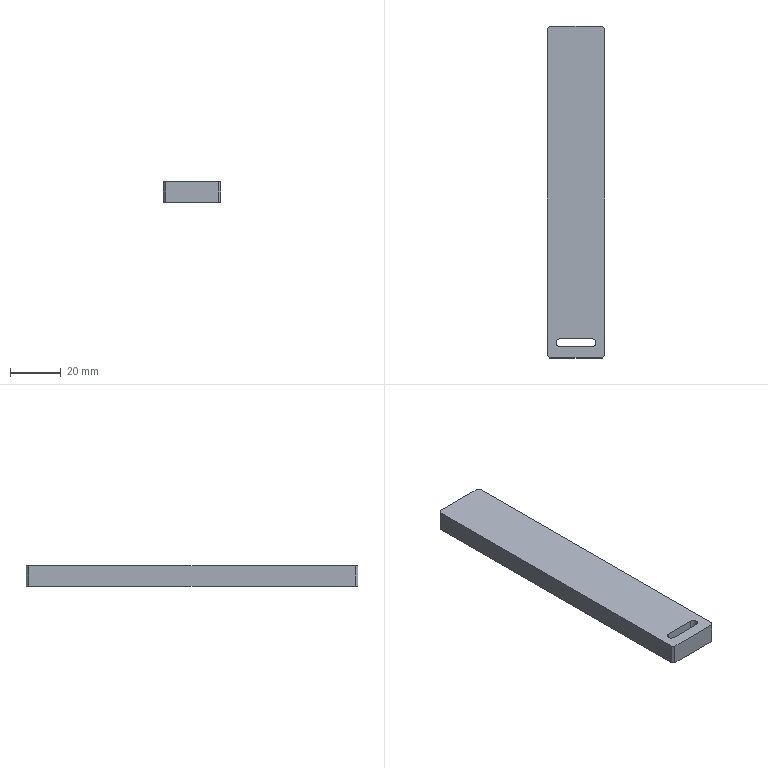Part | STEP file | PN_0029 | 1 solid | 31 faces | box 22.5 x 130.5 x 8 mm | volume 23047 mm3 | plane 12 | cylinder 11 | cone 8 | commonest cylinder face diameters 1.6 x8 3.2 x3